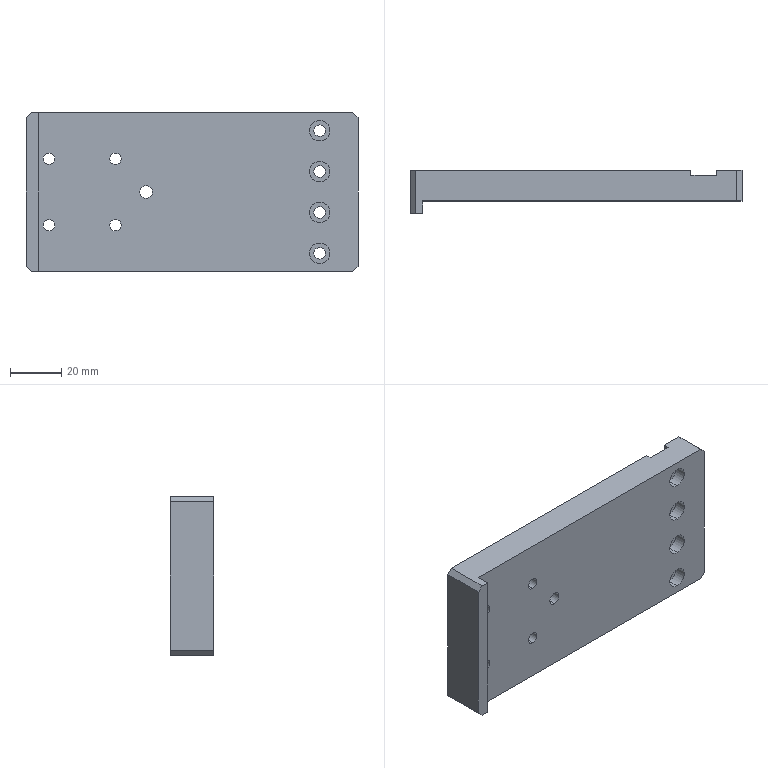Part | SolidWorks | features BaseBody 1 | 1 solid | 58 faces | box 130 x 17 x 62 mm | volume 94014 mm3 | cylinder 34 | plane 24 | commonest cylinder face diameters 4.5 x16 8 x16 5 x2